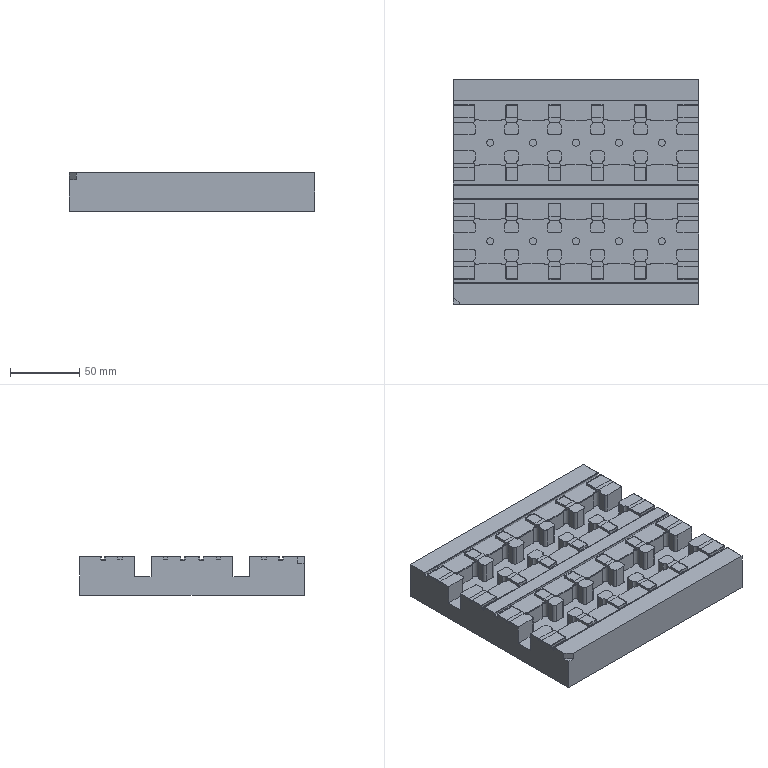NC program | NX | posted by the shop | part box 177 x 162 x 28 mm
Lines 1 to 684 of 240480:
%
O0001
(Machine time: 198.83 MIN)
(===Total Tool:12===)
(T2=D17R0.8FlyCutter D=17.  R=0.8  D-  H02 Z=28.1  )
(T17=C6SpotDrill  D=6.   R=0.   D-  H17 Z=12.45 )
(T15=ZT4.5  D=4.5  DR_a=118 D-  H15 Z=13.5  )
(T10=D10    D=10.  R=0.   D-  H10 Z=13.56 )
(T5=D4      D=4.   R=0.   D5  H05 Z=13.55 )
(T4=D3      D=3.   R=0.   D4  H04 Z=26.22 )
(T11=D10-J  D=10.  R=0.   D-  H11 Z=28.   )
(T3=ZT5.1   D=5.1  DR_a=118 D-  H03 Z=1.35  )
(T14=D4-J   D=4.   R=0.   D-  H14 Z=13.5  )
(T13=D3-J   D=3.   R=0.   D-  H13 Z=26.2  )
(T1=D6ChamferMill   D=6.   R=0.   D-  H01 Z=11.65 )
(T7=D6-J    D=6.   R=0.   D7  H07 Z=23.   )
G80 G90 G17 G49 G40
G91 G28 Z0
M01
N1 T02 M06
(D17R0.8FlyCutter  D=17. R=0.8 H=02 ce=0.20 di=0.10)
(MAX_Z=43. MIN_Z=28.1 Time=10.54M)
T17
G00 G90 G54 X-109. Y78.971 M03 S2000
G43 H02 Z43.
M08
Z32.2
G01 Z30.2 F2500.
X-97.
X95.301
G02 X97. Y77.272 I-.001 J-1.7
G01 Y69.971
G02 X95.47 Y68.441 I-1.53 J0.0
G01 X-95.301
G03 X-97. Y66.742 I.001 J-1.7
G01 Y59.612
G03 X-95.3 Y57.912 I1.7 J0.0
G01 X95.301
G02 X97. Y56.213 I-.001 J-1.7
G01 Y49.082
G02 X95.3 Y47.382 I-1.7 J0.0
G01 X-95.301
G03 X-97. Y45.684 I.001 J-1.7
G01 Y38.553
G03 X-95.3 Y36.853 I1.7 J0.0
G01 X95.301
G02 X97. Y35.154 I-.001 J-1.7
G01 Y28.024
G02 X95.3 Y26.324 I-1.7 J0.0
G01 X-95.301
G03 X-97. Y24.625 I.001 J-1.7
G01 Y17.494
G03 X-95.3 Y15.794 I1.7 J0.0
G01 X95.301
G02 X97. Y14.095 I-.001 J-1.7
G01 Y6.965
G02 X95.3 Y5.265 I-1.7 J0.0
G01 X-95.301
G03 X-97. Y3.566 I.001 J-1.7
G01 Y-3.565
G03 X-95.3 Y-5.265 I1.7 J0.0
G01 X95.301
G02 X97. Y-6.963 I-.001 J-1.7
G01 Y-14.094
G02 X95.3 Y-15.794 I-1.7 J0.0
G01 X-95.301
G03 X-97. Y-17.493 I.001 J-1.7
G01 Y-24.624
G03 X-95.3 Y-26.324 I1.7 J0.0
G01 X95.301
G02 X97. Y-28.022 I-.001 J-1.7
G01 Y-35.153
G02 X95.3 Y-36.853 I-1.7 J0.0
G01 X-95.301
G03 X-97. Y-38.552 I.001 J-1.7
G01 Y-45.682
G03 X-95.3 Y-47.382 I1.7 J0.0
G01 X95.301
G02 X97. Y-49.081 I-.001 J-1.7
G01 Y-56.212
G02 X95.3 Y-57.912 I-1.7 J0.0
G01 X-95.301
G03 X-97. Y-59.611 I.001 J-1.7
G01 Y-66.741
G03 X-95.3 Y-68.441 I1.7 J0.0
G01 X95.301
G02 X97. Y-70.14 I-.001 J-1.7
G01 Y-77.271
G02 X95.3 Y-78.971 I-1.7 J0.0
G01 X-97.
X-109.
Z32.2
G00 Z33.5
Y78.971
Z31.9
G01 Z29.9
X-97.
X95.301
G02 X97. Y77.272 I-.001 J-1.7
G01 Y69.971
G02 X95.47 Y68.441 I-1.53 J0.0
G01 X-95.301
G03 X-97. Y66.742 I.001 J-1.7
G01 Y59.612
G03 X-95.3 Y57.912 I1.7 J0.0
G01 X95.301
G02 X97. Y56.213 I-.001 J-1.7
G01 Y49.082
G02 X95.3 Y47.382 I-1.7 J0.0
G01 X-95.301
G03 X-97. Y45.684 I.001 J-1.7
G01 Y38.553
G03 X-95.3 Y36.853 I1.7 J0.0
G01 X95.301
G02 X97. Y35.154 I-.001 J-1.7
G01 Y28.024
G02 X95.3 Y26.324 I-1.7 J0.0
G01 X-95.301
G03 X-97. Y24.625 I.001 J-1.7
G01 Y17.494
G03 X-95.3 Y15.794 I1.7 J0.0
G01 X95.301
G02 X97. Y14.095 I-.001 J-1.7
G01 Y6.965
G02 X95.3 Y5.265 I-1.7 J0.0
G01 X-95.301
G03 X-97. Y3.566 I.001 J-1.7
G01 Y-3.565
G03 X-95.3 Y-5.265 I1.7 J0.0
G01 X95.301
G02 X97. Y-6.963 I-.001 J-1.7
G01 Y-14.094
G02 X95.3 Y-15.794 I-1.7 J0.0
G01 X-95.301
G03 X-97. Y-17.493 I.001 J-1.7
G01 Y-24.624
G03 X-95.3 Y-26.324 I1.7 J0.0
G01 X95.301
G02 X97. Y-28.022 I-.001 J-1.7
G01 Y-35.153
G02 X95.3 Y-36.853 I-1.7 J0.0
G01 X-95.301
G03 X-97. Y-38.552 I.001 J-1.7
G01 Y-45.682
G03 X-95.3 Y-47.382 I1.7 J0.0
G01 X95.301
G02 X97. Y-49.081 I-.001 J-1.7
G01 Y-56.212
G02 X95.3 Y-57.912 I-1.7 J0.0
G01 X-95.301
G03 X-97. Y-59.611 I.001 J-1.7
G01 Y-66.741
G03 X-95.3 Y-68.441 I1.7 J0.0
G01 X95.301
G02 X97. Y-70.14 I-.001 J-1.7
G01 Y-77.271
G02 X95.3 Y-78.971 I-1.7 J0.0
G01 X-97.
X-109.
Z31.9
G00 Z33.2
Y78.971
Z31.6
G01 Z29.6
X-97.
X95.301
G02 X97. Y77.272 I-.001 J-1.7
G01 Y69.971
G02 X95.47 Y68.441 I-1.53 J0.0
G01 X-95.301
G03 X-97. Y66.742 I.001 J-1.7
G01 Y59.612
G03 X-95.3 Y57.912 I1.7 J0.0
G01 X95.301
G02 X97. Y56.213 I-.001 J-1.7
G01 Y49.082
G02 X95.3 Y47.382 I-1.7 J0.0
G01 X-95.301
G03 X-97. Y45.684 I.001 J-1.7
G01 Y38.553
G03 X-95.3 Y36.853 I1.7 J0.0
G01 X95.301
G02 X97. Y35.154 I-.001 J-1.7
G01 Y28.024
G02 X95.3 Y26.324 I-1.7 J0.0
G01 X-95.301
G03 X-97. Y24.625 I.001 J-1.7
G01 Y17.494
G03 X-95.3 Y15.794 I1.7 J0.0
G01 X95.301
G02 X97. Y14.095 I-.001 J-1.7
G01 Y6.965
G02 X95.3 Y5.265 I-1.7 J0.0
G01 X-95.301
G03 X-97. Y3.566 I.001 J-1.7
G01 Y-3.565
G03 X-95.3 Y-5.265 I1.7 J0.0
G01 X95.301
G02 X97. Y-6.963 I-.001 J-1.7
G01 Y-14.094
G02 X95.3 Y-15.794 I-1.7 J0.0
G01 X-95.301
G03 X-97. Y-17.493 I.001 J-1.7
G01 Y-24.624
G03 X-95.3 Y-26.324 I1.7 J0.0
G01 X95.301
G02 X97. Y-28.022 I-.001 J-1.7
G01 Y-35.153
G02 X95.3 Y-36.853 I-1.7 J0.0
G01 X-95.301
G03 X-97. Y-38.552 I.001 J-1.7
G01 Y-45.682
G03 X-95.3 Y-47.382 I1.7 J0.0
G01 X95.301
G02 X97. Y-49.081 I-.001 J-1.7
G01 Y-56.212
G02 X95.3 Y-57.912 I-1.7 J0.0
G01 X-95.301
G03 X-97. Y-59.611 I.001 J-1.7
G01 Y-66.741
G03 X-95.3 Y-68.441 I1.7 J0.0
G01 X95.301
G02 X97. Y-70.14 I-.001 J-1.7
G01 Y-77.271
G02 X95.3 Y-78.971 I-1.7 J0.0
G01 X-97.
X-109.
Z31.6
G00 Z32.9
Y78.971
Z31.3
G01 Z29.3
X-97.
X95.301
G02 X97. Y77.272 I-.001 J-1.7
G01 Y69.971
G02 X95.47 Y68.441 I-1.53 J0.0
G01 X-95.301
G03 X-97. Y66.742 I.001 J-1.7
G01 Y59.612
G03 X-95.3 Y57.912 I1.7 J0.0
G01 X95.301
G02 X97. Y56.213 I-.001 J-1.7
G01 Y49.082
G02 X95.3 Y47.382 I-1.7 J0.0
G01 X-95.301
G03 X-97. Y45.684 I.001 J-1.7
G01 Y38.553
G03 X-95.3 Y36.853 I1.7 J0.0
G01 X95.301
G02 X97. Y35.154 I-.001 J-1.7
G01 Y28.024
G02 X95.3 Y26.324 I-1.7 J0.0
G01 X-95.301
G03 X-97. Y24.625 I.001 J-1.7
G01 Y17.494
G03 X-95.3 Y15.794 I1.7 J0.0
G01 X95.301
G02 X97. Y14.095 I-.001 J-1.7
G01 Y6.965
G02 X95.3 Y5.265 I-1.7 J0.0
G01 X-95.301
G03 X-97. Y3.566 I.001 J-1.7
G01 Y-3.565
G03 X-95.3 Y-5.265 I1.7 J0.0
G01 X95.301
G02 X97. Y-6.963 I-.001 J-1.7
G01 Y-14.094
G02 X95.3 Y-15.794 I-1.7 J0.0
G01 X-95.301
G03 X-97. Y-17.493 I.001 J-1.7
G01 Y-24.624
G03 X-95.3 Y-26.324 I1.7 J0.0
G01 X95.301
G02 X97. Y-28.022 I-.001 J-1.7
G01 Y-35.153
G02 X95.3 Y-36.853 I-1.7 J0.0
G01 X-95.301
G03 X-97. Y-38.552 I.001 J-1.7
G01 Y-45.682
G03 X-95.3 Y-47.382 I1.7 J0.0
G01 X95.301
G02 X97. Y-49.081 I-.001 J-1.7
G01 Y-56.212
G02 X95.3 Y-57.912 I-1.7 J0.0
G01 X-95.301
G03 X-97. Y-59.611 I.001 J-1.7
G01 Y-66.741
G03 X-95.3 Y-68.441 I1.7 J0.0
G01 X95.301
G02 X97. Y-70.14 I-.001 J-1.7
G01 Y-77.271
G02 X95.3 Y-78.971 I-1.7 J0.0
G01 X-97.
X-109.
Z31.3
G00 Z32.6
Y78.971
Z31.
G01 Z29.
X-97.
X95.301
G02 X97. Y77.272 I-.001 J-1.7
G01 Y69.971
G02 X95.47 Y68.441 I-1.53 J0.0
G01 X-95.301
G03 X-97. Y66.742 I.001 J-1.7
G01 Y59.612
G03 X-95.3 Y57.912 I1.7 J0.0
G01 X95.301
G02 X97. Y56.213 I-.001 J-1.7
G01 Y49.082
G02 X95.3 Y47.382 I-1.7 J0.0
G01 X-95.301
G03 X-97. Y45.684 I.001 J-1.7
G01 Y38.553
G03 X-95.3 Y36.853 I1.7 J0.0
G01 X95.301
G02 X97. Y35.154 I-.001 J-1.7
G01 Y28.024
G02 X95.3 Y26.324 I-1.7 J0.0
G01 X-95.301
G03 X-97. Y24.625 I.001 J-1.7
G01 Y17.494
G03 X-95.3 Y15.794 I1.7 J0.0
G01 X95.301
G02 X97. Y14.095 I-.001 J-1.7
G01 Y6.965
G02 X95.3 Y5.265 I-1.7 J0.0
G01 X-95.301
G03 X-97. Y3.566 I.001 J-1.7
G01 Y-3.565
G03 X-95.3 Y-5.265 I1.7 J0.0
G01 X95.301
G02 X97. Y-6.963 I-.001 J-1.7
G01 Y-14.094
G02 X95.3 Y-15.794 I-1.7 J0.0
G01 X-95.301
G03 X-97. Y-17.493 I.001 J-1.7
G01 Y-24.624
G03 X-95.3 Y-26.324 I1.7 J0.0
G01 X95.301
G02 X97. Y-28.022 I-.001 J-1.7
G01 Y-35.153
G02 X95.3 Y-36.853 I-1.7 J0.0
G01 X-95.301
G03 X-97. Y-38.552 I.001 J-1.7
G01 Y-45.682
G03 X-95.3 Y-47.382 I1.7 J0.0
G01 X95.301
G02 X97. Y-49.081 I-.001 J-1.7
G01 Y-56.212
G02 X95.3 Y-57.912 I-1.7 J0.0
G01 X-95.301
G03 X-97. Y-59.611 I.001 J-1.7
G01 Y-66.741
G03 X-95.3 Y-68.441 I1.7 J0.0
G01 X95.301
G02 X97. Y-70.14 I-.001 J-1.7
G01 Y-77.271
G02 X95.3 Y-78.971 I-1.7 J0.0
G01 X-97.
X-109.
Z31.
G00 Z32.3
Y78.971
Z30.7
G01 Z28.7
X-97.
X95.301
G02 X97. Y77.272 I-.001 J-1.7
G01 Y69.971
G02 X95.47 Y68.441 I-1.53 J0.0
G01 X-95.301
G03 X-97. Y66.742 I.001 J-1.7
G01 Y59.612
G03 X-95.3 Y57.912 I1.7 J0.0
G01 X95.301
G02 X97. Y56.213 I-.001 J-1.7
G01 Y49.082
G02 X95.3 Y47.382 I-1.7 J0.0
G01 X-95.301
G03 X-97. Y45.684 I.001 J-1.7
G01 Y38.553
G03 X-95.3 Y36.853 I1.7 J0.0
G01 X95.301
G02 X97. Y35.154 I-.001 J-1.7
G01 Y28.024
G02 X95.3 Y26.324 I-1.7 J0.0
G01 X-95.301
G03 X-97. Y24.625 I.001 J-1.7
G01 Y17.494
G03 X-95.3 Y15.794 I1.7 J0.0
G01 X95.301
G02 X97. Y14.095 I-.001 J-1.7
G01 Y6.965
G02 X95.3 Y5.265 I-1.7 J0.0
G01 X-95.301
G03 X-97. Y3.566 I.001 J-1.7
G01 Y-3.565
G03 X-95.3 Y-5.265 I1.7 J0.0
G01 X95.301
G02 X97. Y-6.963 I-.001 J-1.7
G01 Y-14.094
G02 X95.3 Y-15.794 I-1.7 J0.0
G01 X-95.301
G03 X-97. Y-17.493 I.001 J-1.7
G01 Y-24.624
G03 X-95.3 Y-26.324 I1.7 J0.0
G01 X95.301
G02 X97. Y-28.022 I-.001 J-1.7
G01 Y-35.153
G02 X95.3 Y-36.853 I-1.7 J0.0
G01 X-95.301
G03 X-97. Y-38.552 I.001 J-1.7
G01 Y-45.682
G03 X-95.3 Y-47.382 I1.7 J0.0
G01 X95.301
G02 X97. Y-49.081 I-.001 J-1.7
G01 Y-56.212
G02 X95.3 Y-57.912 I-1.7 J0.0
G01 X-95.301
G03 X-97. Y-59.611 I.001 J-1.7
G01 Y-66.741
G03 X-95.3 Y-68.441 I1.7 J0.0
G01 X95.301
G02 X97. Y-70.14 I-.001 J-1.7
G01 Y-77.271
G02 X95.3 Y-78.971 I-1.7 J0.0
G01 X-97.
X-109.
Z30.7
G00 Z32.
Y78.971
Z30.4
G01 Z28.4
X-97.
X95.301
G02 X97. Y77.272 I-.001 J-1.7
G01 Y69.971
G02 X95.47 Y68.441 I-1.53 J0.0
G01 X-95.301
G03 X-97. Y66.742 I.001 J-1.7
G01 Y59.612
G03 X-95.3 Y57.912 I1.7 J0.0
G01 X95.301
G02 X97. Y56.213 I-.001 J-1.7
G01 Y49.082
G02 X95.3 Y47.382 I-1.7 J0.0
G01 X-95.301
G03 X-97. Y45.684 I.001 J-1.7
G01 Y38.553
G03 X-95.3 Y36.853 I1.7 J0.0
G01 X95.301
G02 X97. Y35.154 I-.001 J-1.7
G01 Y28.024
G02 X95.3 Y26.324 I-1.7 J0.0
G01 X-95.301
G03 X-97. Y24.625 I.001 J-1.7
G01 Y17.494
G03 X-95.3 Y15.794 I1.7 J0.0
G01 X95.301
G02 X97. Y14.095 I-.001 J-1.7
G01 Y6.965
G02 X95.3 Y5.265 I-1.7 J0.0
G01 X-95.301
G03 X-97. Y3.566 I.001 J-1.7
G01 Y-3.565
G03 X-95.3 Y-5.265 I1.7 J0.0
G01 X95.301
G02 X97. Y-6.963 I-.001 J-1.7
G01 Y-14.094
G02 X95.3 Y-15.794 I-1.7 J0.0
G01 X-95.301
G03 X-97. Y-17.493 I.001 J-1.7
G01 Y-24.624
G03 X-95.3 Y-26.324 I1.7 J0.0
G01 X95.301
G02 X97. Y-28.022 I-.001 J-1.7
G01 Y-35.153
G02 X95.3 Y-36.853 I-1.7 J0.0
G01 X-95.301
G03 X-97. Y-38.552 I.001 J-1.7
G01 Y-45.682
G03 X-95.3 Y-47.382 I1.7 J0.0
G01 X95.301
G02 X97. Y-49.081 I-.001 J-1.7
G01 Y-56.212
G02 X95.3 Y-57.912 I-1.7 J0.0
G01 X-95.301
G03 X-97. Y-59.611 I.001 J-1.7
G01 Y-66.741
G03 X-95.3 Y-68.441 I1.7 J0.0
G01 X95.301
G02 X97. Y-70.14 I-.001 J-1.7
G01 Y-77.271
G02 X95.3 Y-78.971 I-1.7 J0.0
G01 X-97.
X-109.
Z30.4
G00 Z31.7
Y78.971
Z30.1
G01 Z28.1
X-97.
X95.301
G02 X97. Y77.272 I-.001 J-1.7
G01 Y69.971
G02 X95.47 Y68.441 I-1.53 J0.0
G01 X-95.301
G03 X-97. Y66.742 I.001 J-1.7
G01 Y59.612
G03 X-95.3 Y57.912 I1.7 J0.0
G01 X95.301
G02 X97. Y56.213 I-.001 J-1.7
G01 Y49.082
G02 X95.3 Y47.382 I-1.7 J0.0
G01 X-95.301
G03 X-97. Y45.684 I.001 J-1.7
G01 Y38.553
G03 X-95.3 Y36.853 I1.7 J0.0
G01 X95.301
G02 X97. Y35.154 I-.001 J-1.7
G01 Y28.024
G02 X95.3 Y26.324 I-1.7 J0.0
G01 X-95.301
G03 X-97. Y24.625 I.001 J-1.7
G01 Y17.494
G03 X-95.3 Y15.794 I1.7 J0.0
G01 X95.301
G02 X97. Y14.095 I-.001 J-1.7
G01 Y6.965
G02 X95.3 Y5.265 I-1.7 J0.0
G01 X-95.301
G03 X-97. Y3.566 I.001 J-1.7
G01 Y-3.565
G03 X-95.3 Y-5.265 I1.7 J0.0
G01 X95.301
G02 X97. Y-6.963 I-.001 J-1.7
G01 Y-14.094
G02 X95.3 Y-15.794 I-1.7 J0.0
G01 X-95.301
G03 X-97. Y-17.493 I.001 J-1.7
G01 Y-24.624
G03 X-95.3 Y-26.324 I1.7 J0.0
G01 X95.301
G02 X97. Y-28.022 I-.001 J-1.7
G01 Y-35.153
G02 X95.3 Y-36.853 I-1.7 J0.0
G01 X-95.301
G03 X-97. Y-38.552 I.001 J-1.7
G01 Y-45.682
G03 X-95.3 Y-47.382 I1.7 J0.0
G01 X95.301
G02 X97. Y-49.081 I-.001 J-1.7
G01 Y-56.212
G02 X95.3 Y-57.912 I-1.7 J0.0
G01 X-95.301
G03 X-97. Y-59.611 I.001 J-1.7
G01 Y-66.741
G03 X-95.3 Y-68.441 I1.7 J0.0
G01 X95.301
G02 X97. Y-70.14 I-.001 J-1.7
G01 Y-77.271
G02 X95.3 Y-78.971 I-1.7 J0.0
G01 X-97.
X-109.
Z30.1
G00 Z43.
G91 G28 Z0.0
M05
M09
G91 G28 Z0.0
M01
N2 T17 M06
(C6SpotDrill  D=6. R=0. H=17 ce=0.00 di=0.10)
(MAX_Z=43. MIN_Z=27.2 Time=1.50M)
T15
G00 G90 G54 X-71.477 Y50.097 M03 S1500
G43 H17 Z43.
M08
G98 G81 X-71.477 Y50.097 Z27.2 R29. F50.
X-52.523
X-40.477
X-21.523
X-9.477
X9.477
X21.523
X40.477
X52.523
X71.477
Y21.103
X52.523
X40.477
X21.523
X9.477
X-9.477
X-21.523
X-40.477
X-52.523
X-71.477
Y-21.103
X-52.523
X-40.477
X-21.523
X-9.477
X9.477
X21.523
X40.477
X52.523
X71.477
Y-50.097
X52.523
X40.477
X21.523
X9.477
X-9.477
X-21.523
X-40.477
X-52.523
X-71.477
G80
G00 Z43.
G91 G28 Z0.0
M05
M09
G91 G28 Z0.0
M01
N3 T15 M06
(ZT4.5 D=4.5 DR_a=118 H=15)
(MAX_Z=43. MIN_Z=13.5 Time=12.46M)
T10
G00 G90 G54 X-71.477 Y50.097 M03 S1000
G43 H15 Z43.
M08
G98 G83 X-71.477 Y50.097 Z13.5 R29. F50. Q1.
X-52.523
X-40.477
X-21.523
X-9.477
X9.477
X21.523
X40.477
X52.523
X71.477
Y21.103
X52.523
X40.477
X21.523
X9.477
X-9.477
X-21.523
X-40.477
X-52.523
X-71.477
Y-21.103
X-52.523
X-40.477
X-21.523
X-9.477
X9.477
X21.523
X40.477
X52.523
X71.477
Y-50.097
X52.523
X40.477
X21.523
X9.477
X-9.477
X-21.523
X-40.477
X-52.523
X-71.477
G80
G00 Z43.
G91 G28 Z0.0
M05
M09
G91 G28 Z0.0
M01